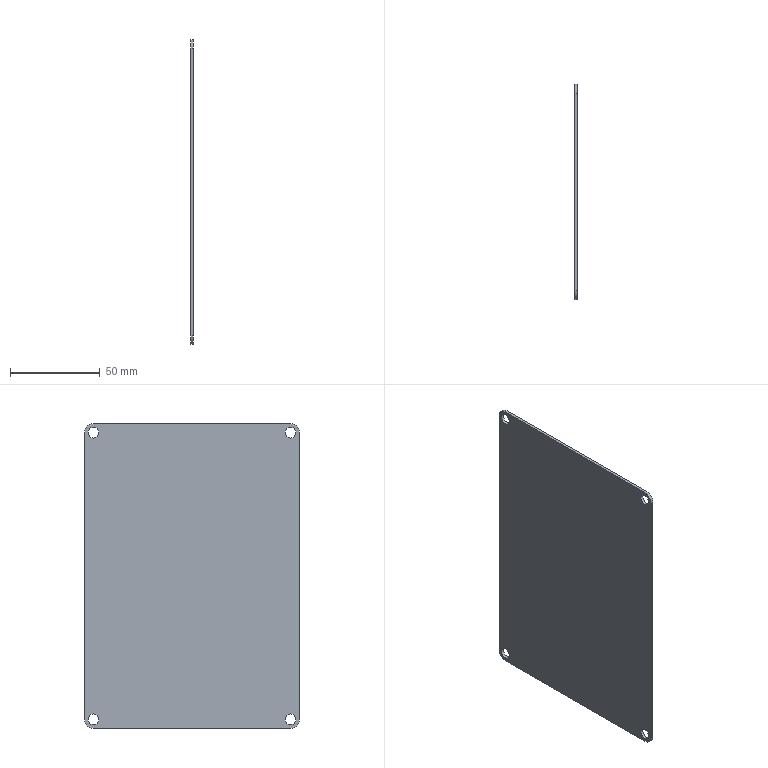Part | SolidWorks | 1 solid | 18 faces | box 1.5 x 120 x 170 mm | volume 30398 mm3 | cylinder 12 | plane 6 | commonest cylinder face diameters 6 x8 10 x4
STEP:
#1=CARTESIAN_POINT('',(-1.5,-55.,77.));
#2=VERTEX_POINT('',#1);
#3=CARTESIAN_POINT('',(-1.5,-55.,83.));
#4=VERTEX_POINT('',#3);
#5=CARTESIAN_POINT('',(-1.5,-55.,80.));
#6=DIRECTION('',(-1.,0.,0.));
#7=DIRECTION('',(0.,0.,-1.));
#8=AXIS2_PLACEMENT_3D('',#5,#6,#7);
#9=CIRCLE('',#8,3.);
#10=EDGE_CURVE('',#2,#4,#9,.T.);
#11=ORIENTED_EDGE('',*,*,#10,.T.);
#12=CARTESIAN_POINT('',(0.,-55.,83.));
#13=VERTEX_POINT('',#12);
#14=CARTESIAN_POINT('',(-1.501,-55.,83.));
#15=DIRECTION('',(1.,0.,0.));
#16=VECTOR('',#15,1000.);
#17=LINE('',#14,#16);
#18=EDGE_CURVE('',#4,#13,#17,.T.);
#19=ORIENTED_EDGE('',*,*,#18,.T.);
#20=CARTESIAN_POINT('',(0.,-55.,77.));
#21=VERTEX_POINT('',#20);
#22=CARTESIAN_POINT('',(0.,-55.,80.));
#23=DIRECTION('',(1.,0.,0.));
#24=DIRECTION('',(0.,0.,-1.));
#25=AXIS2_PLACEMENT_3D('',#22,#23,#24);
#26=CIRCLE('',#25,3.);
#27=EDGE_CURVE('',#13,#21,#26,.T.);
#28=ORIENTED_EDGE('',*,*,#27,.T.);
#29=CARTESIAN_POINT('',(-1.501,-55.,77.));
#30=DIRECTION('',(1.,0.,0.));
#31=VECTOR('',#30,1000.);
#32=LINE('',#29,#31);
#33=EDGE_CURVE('',#2,#21,#32,.T.);
#34=ORIENTED_EDGE('',*,*,#33,.F.);
#35=EDGE_LOOP('',(#11,#19,#28,#34));
#36=FACE_OUTER_BOUND('',#35,.T.);
#37=CARTESIAN_POINT('',(-1.501,-55.,80.));
#38=DIRECTION('',(1.,0.,0.));
#39=DIRECTION('',(0.,0.,-1.));
#40=AXIS2_PLACEMENT_3D('',#37,#38,#39);
#41=CYLINDRICAL_SURFACE('',#40,3.);
#42=ADVANCED_FACE('',(#36),#41,.F.);
#43=CARTESIAN_POINT('',(-1.5,-55.,-83.));
#44=VERTEX_POINT('',#43);
#45=CARTESIAN_POINT('',(-1.5,-55.,-77.));
#46=VERTEX_POINT('',#45);
#47=CARTESIAN_POINT('',(-1.5,-55.,-80.));
#48=DIRECTION('',(-1.,0.,0.));
#49=DIRECTION('',(0.,0.,-1.));
#50=AXIS2_PLACEMENT_3D('',#47,#48,#49);
#51=CIRCLE('',#50,3.);
#52=EDGE_CURVE('',#44,#46,#51,.T.);
#53=ORIENTED_EDGE('',*,*,#52,.T.);
#54=CARTESIAN_POINT('',(0.,-55.,-77.));
#55=VERTEX_POINT('',#54);
#56=CARTESIAN_POINT('',(-1.501,-55.,-77.));
#57=DIRECTION('',(1.,0.,0.));
#58=VECTOR('',#57,1000.);
#59=LINE('',#56,#58);
#60=EDGE_CURVE('',#46,#55,#59,.T.);
#61=ORIENTED_EDGE('',*,*,#60,.T.);
#62=CARTESIAN_POINT('',(0.,-55.,-83.));
#63=VERTEX_POINT('',#62);
#64=CARTESIAN_POINT('',(0.,-55.,-80.));
#65=DIRECTION('',(1.,0.,0.));
#66=DIRECTION('',(0.,0.,-1.));
#67=AXIS2_PLACEMENT_3D('',#64,#65,#66);
#68=CIRCLE('',#67,3.);
#69=EDGE_CURVE('',#55,#63,#68,.T.);
#70=ORIENTED_EDGE('',*,*,#69,.T.);
#71=CARTESIAN_POINT('',(-1.501,-55.,-83.));
#72=DIRECTION('',(1.,0.,0.));
#73=VECTOR('',#72,1000.);
#74=LINE('',#71,#73);
#75=EDGE_CURVE('',#44,#63,#74,.T.);
#76=ORIENTED_EDGE('',*,*,#75,.F.);
#77=EDGE_LOOP('',(#53,#61,#70,#76));
#78=FACE_OUTER_BOUND('',#77,.T.);
#79=CARTESIAN_POINT('',(-1.501,-55.,-80.));
#80=DIRECTION('',(1.,0.,0.));
#81=DIRECTION('',(0.,0.,-1.));
#82=AXIS2_PLACEMENT_3D('',#79,#80,#81);
#83=CYLINDRICAL_SURFACE('',#82,3.);
#84=ADVANCED_FACE('',(#78),#83,.F.);
#85=CARTESIAN_POINT('',(-1.5,55.,-83.));
#86=VERTEX_POINT('',#85);
#87=CARTESIAN_POINT('',(-1.5,55.,-77.));
#88=VERTEX_POINT('',#87);
#89=CARTESIAN_POINT('',(-1.5,55.,-80.));
#90=DIRECTION('',(-1.,0.,0.));
#91=DIRECTION('',(0.,0.,-1.));
#92=AXIS2_PLACEMENT_3D('',#89,#90,#91);
#93=CIRCLE('',#92,3.);
#94=EDGE_CURVE('',#86,#88,#93,.T.);
#95=ORIENTED_EDGE('',*,*,#94,.T.);
#96=CARTESIAN_POINT('',(0.,55.,-77.));
#97=VERTEX_POINT('',#96);
#98=CARTESIAN_POINT('',(-1.501,55.,-77.));
#99=DIRECTION('',(1.,0.,0.));
#100=VECTOR('',#99,1000.);
#101=LINE('',#98,#100);
#102=EDGE_CURVE('',#88,#97,#101,.T.);
#103=ORIENTED_EDGE('',*,*,#102,.T.);
#104=CARTESIAN_POINT('',(0.,55.,-83.));
#105=VERTEX_POINT('',#104);
#106=CARTESIAN_POINT('',(0.,55.,-80.));
#107=DIRECTION('',(1.,0.,0.));
#108=DIRECTION('',(0.,0.,-1.));
#109=AXIS2_PLACEMENT_3D('',#106,#107,#108);
#110=CIRCLE('',#109,3.);
#111=EDGE_CURVE('',#97,#105,#110,.T.);
#112=ORIENTED_EDGE('',*,*,#111,.T.);
#113=CARTESIAN_POINT('',(-1.501,55.,-83.));
#114=DIRECTION('',(1.,0.,0.));
#115=VECTOR('',#114,1000.);
#116=LINE('',#113,#115);
#117=EDGE_CURVE('',#86,#105,#116,.T.);
#118=ORIENTED_EDGE('',*,*,#117,.F.);
#119=EDGE_LOOP('',(#95,#103,#112,#118));
#120=FACE_OUTER_BOUND('',#119,.T.);
#121=CARTESIAN_POINT('',(-1.501,55.,-80.));
#122=DIRECTION('',(1.,0.,0.));
#123=DIRECTION('',(0.,0.,-1.));
#124=AXIS2_PLACEMENT_3D('',#121,#122,#123);
#125=CYLINDRICAL_SURFACE('',#124,3.);
#126=ADVANCED_FACE('',(#120),#125,.F.);
#127=CARTESIAN_POINT('',(-1.5,55.,77.));
#128=VERTEX_POINT('',#127);
#129=CARTESIAN_POINT('',(-1.5,55.,83.));
#130=VERTEX_POINT('',#129);
#131=CARTESIAN_POINT('',(-1.5,55.,80.));
#132=DIRECTION('',(-1.,0.,0.));
#133=DIRECTION('',(0.,0.,-1.));
#134=AXIS2_PLACEMENT_3D('',#131,#132,#133);
#135=CIRCLE('',#134,3.);
#136=EDGE_CURVE('',#128,#130,#135,.T.);
#137=ORIENTED_EDGE('',*,*,#136,.T.);
#138=CARTESIAN_POINT('',(0.,55.,83.));
#139=VERTEX_POINT('',#138);
#140=CARTESIAN_POINT('',(-1.501,55.,83.));
#141=DIRECTION('',(1.,0.,0.));
#142=VECTOR('',#141,1000.);
#143=LINE('',#140,#142);
#144=EDGE_CURVE('',#130,#139,#143,.T.);
#145=ORIENTED_EDGE('',*,*,#144,.T.);
#146=CARTESIAN_POINT('',(0.,55.,77.));
#147=VERTEX_POINT('',#146);
#148=CARTESIAN_POINT('',(0.,55.,80.));
#149=DIRECTION('',(1.,0.,0.));
#150=DIRECTION('',(0.,0.,-1.));
#151=AXIS2_PLACEMENT_3D('',#148,#149,#150);
#152=CIRCLE('',#151,3.);
#153=EDGE_CURVE('',#139,#147,#152,.T.);
#154=ORIENTED_EDGE('',*,*,#153,.T.);
#155=CARTESIAN_POINT('',(-1.501,55.,77.));
#156=DIRECTION('',(1.,0.,0.));
#157=VECTOR('',#156,1000.);
#158=LINE('',#155,#157);
#159=EDGE_CURVE('',#128,#147,#158,.T.);
#160=ORIENTED_EDGE('',*,*,#159,.F.);
#161=EDGE_LOOP('',(#137,#145,#154,#160));
#162=FACE_OUTER_BOUND('',#161,.T.);
#163=CARTESIAN_POINT('',(-1.501,55.,80.));
#164=DIRECTION('',(1.,0.,0.));
#165=DIRECTION('',(0.,0.,-1.));
#166=AXIS2_PLACEMENT_3D('',#163,#164,#165);
#167=CYLINDRICAL_SURFACE('',#166,3.);
#168=ADVANCED_FACE('',(#162),#167,.F.);
#169=CARTESIAN_POINT('',(-1.5,55.,85.));
#170=VERTEX_POINT('',#169);
#171=CARTESIAN_POINT('',(-1.5,-55.,85.));
#172=VERTEX_POINT('',#171);
#173=CARTESIAN_POINT('',(-1.5,-60.,85.));
#174=DIRECTION('',(0.,-1.,0.));
#175=VECTOR('',#174,1000.);
#176=LINE('',#173,#175);
#177=EDGE_CURVE('',#170,#172,#176,.T.);
#178=ORIENTED_EDGE('',*,*,#177,.T.);
#179=CARTESIAN_POINT('',(0.,-55.,85.));
#180=VERTEX_POINT('',#179);
#181=CARTESIAN_POINT('',(-1.5,-55.,85.));
#182=DIRECTION('',(1.,0.,0.));
#183=VECTOR('',#182,1000.);
#184=LINE('',#181,#183);
#185=EDGE_CURVE('',#172,#180,#184,.T.);
#186=ORIENTED_EDGE('',*,*,#185,.T.);
#187=CARTESIAN_POINT('',(0.,55.,85.));
#188=VERTEX_POINT('',#187);
#189=CARTESIAN_POINT('',(0.,-60.,85.));
#190=DIRECTION('',(0.,-1.,0.));
#191=VECTOR('',#190,1000.);
#192=LINE('',#189,#191);
#193=EDGE_CURVE('',#188,#180,#192,.T.);
#194=ORIENTED_EDGE('',*,*,#193,.F.);
#195=CARTESIAN_POINT('',(-1.5,55.,85.));
#196=DIRECTION('',(-1.,0.,0.));
#197=VECTOR('',#196,1000.);
#198=LINE('',#195,#197);
#199=EDGE_CURVE('',#188,#170,#198,.T.);
#200=ORIENTED_EDGE('',*,*,#199,.T.);
#201=EDGE_LOOP('',(#178,#186,#194,#200));
#202=FACE_OUTER_BOUND('',#201,.T.);
#203=CARTESIAN_POINT('',(-1.5,-60.,85.));
#204=DIRECTION('',(0.,0.,1.));
#205=DIRECTION('',(0.,-1.,0.));
#206=AXIS2_PLACEMENT_3D('',#203,#204,#205);
#207=PLANE('',#206);
#208=ADVANCED_FACE('',(#202),#207,.T.);
#209=CARTESIAN_POINT('',(0.,60.,-80.));
#210=VERTEX_POINT('',#209);
#211=CARTESIAN_POINT('',(0.,60.,80.));
#212=VERTEX_POINT('',#211);
#213=CARTESIAN_POINT('',(0.,60.,-85.));
#214=DIRECTION('',(0.,0.,1.));
#215=VECTOR('',#214,1000.);
#216=LINE('',#213,#215);
#217=EDGE_CURVE('',#210,#212,#216,.T.);
#218=ORIENTED_EDGE('',*,*,#217,.F.);
#219=CARTESIAN_POINT('',(-1.5,60.,-80.));
#220=VERTEX_POINT('',#219);
#221=CARTESIAN_POINT('',(-1.5,60.,-80.));
#222=DIRECTION('',(-1.,0.,0.));
#223=VECTOR('',#222,1000.);
#224=LINE('',#221,#223);
#225=EDGE_CURVE('',#210,#220,#224,.T.);
#226=ORIENTED_EDGE('',*,*,#225,.T.);
#227=CARTESIAN_POINT('',(-1.5,60.,80.));
#228=VERTEX_POINT('',#227);
#229=CARTESIAN_POINT('',(-1.5,60.,-85.));
#230=DIRECTION('',(0.,0.,1.));
#231=VECTOR('',#230,1000.);
#232=LINE('',#229,#231);
#233=EDGE_CURVE('',#220,#228,#232,.T.);
#234=ORIENTED_EDGE('',*,*,#233,.T.);
#235=CARTESIAN_POINT('',(-1.5,60.,80.));
#236=DIRECTION('',(1.,0.,0.));
#237=VECTOR('',#236,1000.);
#238=LINE('',#235,#237);
#239=EDGE_CURVE('',#228,#212,#238,.T.);
#240=ORIENTED_EDGE('',*,*,#239,.T.);
#241=EDGE_LOOP('',(#218,#226,#234,#240));
#242=FACE_OUTER_BOUND('',#241,.T.);
#243=CARTESIAN_POINT('',(-1.5,60.,-85.));
#244=DIRECTION('',(0.,1.,0.));
#245=DIRECTION('',(0.,0.,1.));
#246=AXIS2_PLACEMENT_3D('',#243,#244,#245);
#247=PLANE('',#246);
#248=ADVANCED_FACE('',(#242),#247,.T.);
#249=CARTESIAN_POINT('',(0.,-55.,-85.));
#250=VERTEX_POINT('',#249);
#251=CARTESIAN_POINT('',(0.,55.,-85.));
#252=VERTEX_POINT('',#251);
#253=CARTESIAN_POINT('',(0.,-60.,-85.));
#254=DIRECTION('',(0.,1.,0.));
#255=VECTOR('',#254,1000.);
#256=LINE('',#253,#255);
#257=EDGE_CURVE('',#250,#252,#256,.T.);
#258=ORIENTED_EDGE('',*,*,#257,.F.);
#259=CARTESIAN_POINT('',(-1.5,-55.,-85.));
#260=VERTEX_POINT('',#259);
#261=CARTESIAN_POINT('',(-1.5,-55.,-85.));
#262=DIRECTION('',(-1.,0.,0.));
#263=VECTOR('',#262,1000.);
#264=LINE('',#261,#263);
#265=EDGE_CURVE('',#250,#260,#264,.T.);
#266=ORIENTED_EDGE('',*,*,#265,.T.);
#267=CARTESIAN_POINT('',(-1.5,55.,-85.));
#268=VERTEX_POINT('',#267);
#269=CARTESIAN_POINT('',(-1.5,-60.,-85.));
#270=DIRECTION('',(0.,1.,0.));
#271=VECTOR('',#270,1000.);
#272=LINE('',#269,#271);
#273=EDGE_CURVE('',#260,#268,#272,.T.);
#274=ORIENTED_EDGE('',*,*,#273,.T.);
#275=CARTESIAN_POINT('',(-1.5,55.,-85.));
#276=DIRECTION('',(1.,0.,0.));
#277=VECTOR('',#276,1000.);
#278=LINE('',#275,#277);
#279=EDGE_CURVE('',#268,#252,#278,.T.);
#280=ORIENTED_EDGE('',*,*,#279,.T.);
#281=EDGE_LOOP('',(#258,#266,#274,#280));
#282=FACE_OUTER_BOUND('',#281,.T.);
#283=CARTESIAN_POINT('',(-1.5,-60.,-85.));
#284=DIRECTION('',(0.,0.,-1.));
#285=DIRECTION('',(-1.,0.,0.));
#286=AXIS2_PLACEMENT_3D('',#283,#284,#285);
#287=PLANE('',#286);
#288=ADVANCED_FACE('',(#282),#287,.T.);
#289=CARTESIAN_POINT('',(0.,-60.,80.));
#290=VERTEX_POINT('',#289);
#291=CARTESIAN_POINT('',(0.,-60.,-80.));
#292=VERTEX_POINT('',#291);
#293=CARTESIAN_POINT('',(0.,-60.,-85.));
#294=DIRECTION('',(0.,0.,-1.));
#295=VECTOR('',#294,1000.);
#296=LINE('',#293,#295);
#297=EDGE_CURVE('',#290,#292,#296,.T.);
#298=ORIENTED_EDGE('',*,*,#297,.F.);
#299=CARTESIAN_POINT('',(-1.5,-60.,80.));
#300=VERTEX_POINT('',#299);
#301=CARTESIAN_POINT('',(-1.5,-60.,80.));
#302=DIRECTION('',(-1.,0.,0.));
#303=VECTOR('',#302,1000.);
#304=LINE('',#301,#303);
#305=EDGE_CURVE('',#290,#300,#304,.T.);
#306=ORIENTED_EDGE('',*,*,#305,.T.);
#307=CARTESIAN_POINT('',(-1.5,-60.,-80.));
#308=VERTEX_POINT('',#307);
#309=CARTESIAN_POINT('',(-1.5,-60.,-85.));
#310=DIRECTION('',(0.,0.,-1.));
#311=VECTOR('',#310,1000.);
#312=LINE('',#309,#311);
#313=EDGE_CURVE('',#300,#308,#312,.T.);
#314=ORIENTED_EDGE('',*,*,#313,.T.);
#315=CARTESIAN_POINT('',(-1.5,-60.,-80.));
#316=DIRECTION('',(1.,0.,0.));
#317=VECTOR('',#316,1000.);
#318=LINE('',#315,#317);
#319=EDGE_CURVE('',#308,#292,#318,.T.);
#320=ORIENTED_EDGE('',*,*,#319,.T.);
#321=EDGE_LOOP('',(#298,#306,#314,#320));
#322=FACE_OUTER_BOUND('',#321,.T.);
#323=CARTESIAN_POINT('',(-1.5,-60.,-85.));
#324=DIRECTION('',(0.,-1.,0.));
#325=DIRECTION('',(0.,0.,-1.));
#326=AXIS2_PLACEMENT_3D('',#323,#324,#325);
#327=PLANE('',#326);
#328=ADVANCED_FACE('',(#322),#327,.T.);
#329=ORIENTED_EDGE('',*,*,#10,.F.);
#330=CARTESIAN_POINT('',(-1.5,-55.,80.));
#331=DIRECTION('',(-1.,0.,0.));
#332=DIRECTION('',(0.,0.,-1.));
#333=AXIS2_PLACEMENT_3D('',#330,#331,#332);
#334=CIRCLE('',#333,3.);
#335=EDGE_CURVE('',#4,#2,#334,.T.);
#336=ORIENTED_EDGE('',*,*,#335,.F.);
#337=EDGE_LOOP('',(#329,#336));
#338=FACE_BOUND('',#337,.T.);
#339=ORIENTED_EDGE('',*,*,#52,.F.);
#340=CARTESIAN_POINT('',(-1.5,-55.,-80.));
#341=DIRECTION('',(-1.,0.,0.));
#342=DIRECTION('',(0.,0.,-1.));
#343=AXIS2_PLACEMENT_3D('',#340,#341,#342);
#344=CIRCLE('',#343,3.);
#345=EDGE_CURVE('',#46,#44,#344,.T.);
#346=ORIENTED_EDGE('',*,*,#345,.F.);
#347=EDGE_LOOP('',(#339,#346));
#348=FACE_BOUND('',#347,.T.);
#349=ORIENTED_EDGE('',*,*,#94,.F.);
#350=CARTESIAN_POINT('',(-1.5,55.,-80.));
#351=DIRECTION('',(-1.,0.,0.));
#352=DIRECTION('',(0.,0.,-1.));
#353=AXIS2_PLACEMENT_3D('',#350,#351,#352);
#354=CIRCLE('',#353,3.);
#355=EDGE_CURVE('',#88,#86,#354,.T.);
#356=ORIENTED_EDGE('',*,*,#355,.F.);
#357=EDGE_LOOP('',(#349,#356));
#358=FACE_BOUND('',#357,.T.);
#359=ORIENTED_EDGE('',*,*,#136,.F.);
#360=CARTESIAN_POINT('',(-1.5,55.,80.));
#361=DIRECTION('',(-1.,0.,0.));
#362=DIRECTION('',(0.,0.,-1.));
#363=AXIS2_PLACEMENT_3D('',#360,#361,#362);
#364=CIRCLE('',#363,3.);
#365=EDGE_CURVE('',#130,#128,#364,.T.);
#366=ORIENTED_EDGE('',*,*,#365,.F.);
#367=EDGE_LOOP('',(#359,#366));
#368=FACE_BOUND('',#367,.T.);
#369=ORIENTED_EDGE('',*,*,#313,.F.);
#370=CARTESIAN_POINT('',(-1.5,-55.,80.));
#371=DIRECTION('',(-1.,0.,0.));
#372=DIRECTION('',(0.,0.,-1.));
#373=AXIS2_PLACEMENT_3D('',#370,#371,#372);
#374=CIRCLE('',#373,5.);
#375=EDGE_CURVE('',#300,#172,#374,.T.);
#376=ORIENTED_EDGE('',*,*,#375,.T.);
#377=ORIENTED_EDGE('',*,*,#177,.F.);
#378=CARTESIAN_POINT('',(-1.5,55.,80.));
#379=DIRECTION('',(-1.,0.,0.));
#380=DIRECTION('',(0.,0.,-1.));
#381=AXIS2_PLACEMENT_3D('',#378,#379,#380);
#382=CIRCLE('',#381,5.);
#383=EDGE_CURVE('',#170,#228,#382,.T.);
#384=ORIENTED_EDGE('',*,*,#383,.T.);
#385=ORIENTED_EDGE('',*,*,#233,.F.);
#386=CARTESIAN_POINT('',(-1.5,55.,-80.));
#387=DIRECTION('',(-1.,0.,0.));
#388=DIRECTION('',(0.,0.,-1.));
#389=AXIS2_PLACEMENT_3D('',#386,#387,#388);
#390=CIRCLE('',#389,5.);
#391=EDGE_CURVE('',#220,#268,#390,.T.);
#392=ORIENTED_EDGE('',*,*,#391,.T.);
#393=ORIENTED_EDGE('',*,*,#273,.F.);
#394=CARTESIAN_POINT('',(-1.5,-55.,-80.));
#395=DIRECTION('',(-1.,0.,0.));
#396=DIRECTION('',(0.,0.,-1.));
#397=AXIS2_PLACEMENT_3D('',#394,#395,#396);
#398=CIRCLE('',#397,5.);
#399=EDGE_CURVE('',#260,#308,#398,.T.);
#400=ORIENTED_EDGE('',*,*,#399,.T.);
#401=EDGE_LOOP('',(#369,#376,#377,#384,#385,#392,#393,#400));
#402=FACE_OUTER_BOUND('',#401,.T.);
#403=CARTESIAN_POINT('',(-1.5,0.,0.));
#404=DIRECTION('',(1.,0.,0.));
#405=DIRECTION('',(0.,0.,-1.));
#406=AXIS2_PLACEMENT_3D('',#403,#404,#405);
#407=PLANE('',#406);
#408=ADVANCED_FACE('',(#338,#348,#358,#368,#402),#407,.F.);
#409=CARTESIAN_POINT('',(0.,-55.,80.));
#410=DIRECTION('',(1.,0.,0.));
#411=DIRECTION('',(0.,0.,-1.));
#412=AXIS2_PLACEMENT_3D('',#409,#410,#411);
#413=CIRCLE('',#412,3.);
#414=EDGE_CURVE('',#21,#13,#413,.T.);
#415=ORIENTED_EDGE('',*,*,#414,.F.);
#416=ORIENTED_EDGE('',*,*,#27,.F.);
#417=EDGE_LOOP('',(#415,#416));
#418=FACE_BOUND('',#417,.T.);
#419=CARTESIAN_POINT('',(0.,-55.,-80.));
#420=DIRECTION('',(1.,0.,0.));
#421=DIRECTION('',(0.,0.,-1.));
#422=AXIS2_PLACEMENT_3D('',#419,#420,#421);
#423=CIRCLE('',#422,3.);
#424=EDGE_CURVE('',#63,#55,#423,.T.);
#425=ORIENTED_EDGE('',*,*,#424,.F.);
#426=ORIENTED_EDGE('',*,*,#69,.F.);
#427=EDGE_LOOP('',(#425,#426));
#428=FACE_BOUND('',#427,.T.);
#429=CARTESIAN_POINT('',(0.,55.,-80.));
#430=DIRECTION('',(1.,0.,0.));
#431=DIRECTION('',(0.,0.,-1.));
#432=AXIS2_PLACEMENT_3D('',#429,#430,#431);
#433=CIRCLE('',#432,3.);
#434=EDGE_CURVE('',#105,#97,#433,.T.);
#435=ORIENTED_EDGE('',*,*,#434,.F.);
#436=ORIENTED_EDGE('',*,*,#111,.F.);
#437=EDGE_LOOP('',(#435,#436));
#438=FACE_BOUND('',#437,.T.);
#439=CARTESIAN_POINT('',(0.,55.,80.));
#440=DIRECTION('',(1.,0.,0.));
#441=DIRECTION('',(0.,0.,-1.));
#442=AXIS2_PLACEMENT_3D('',#439,#440,#441);
#443=CIRCLE('',#442,3.);
#444=EDGE_CURVE('',#147,#139,#443,.T.);
#445=ORIENTED_EDGE('',*,*,#444,.F.);
#446=ORIENTED_EDGE('',*,*,#153,.F.);
#447=EDGE_LOOP('',(#445,#446));
#448=FACE_BOUND('',#447,.T.);
#449=ORIENTED_EDGE('',*,*,#193,.T.);
#450=CARTESIAN_POINT('',(0.,-55.,80.));
#451=DIRECTION('',(1.,0.,0.));
#452=DIRECTION('',(0.,0.,-1.));
#453=AXIS2_PLACEMENT_3D('',#450,#451,#452);
#454=CIRCLE('',#453,5.);
#455=EDGE_CURVE('',#180,#290,#454,.T.);
#456=ORIENTED_EDGE('',*,*,#455,.T.);
#457=ORIENTED_EDGE('',*,*,#297,.T.);
#458=CARTESIAN_POINT('',(0.,-55.,-80.));
#459=DIRECTION('',(1.,0.,0.));
#460=DIRECTION('',(0.,0.,-1.));
#461=AXIS2_PLACEMENT_3D('',#458,#459,#460);
#462=CIRCLE('',#461,5.);
#463=EDGE_CURVE('',#292,#250,#462,.T.);
#464=ORIENTED_EDGE('',*,*,#463,.T.);
#465=ORIENTED_EDGE('',*,*,#257,.T.);
#466=CARTESIAN_POINT('',(0.,55.,-80.));
#467=DIRECTION('',(1.,0.,0.));
#468=DIRECTION('',(0.,0.,-1.));
#469=AXIS2_PLACEMENT_3D('',#466,#467,#468);
#470=CIRCLE('',#469,5.);
#471=EDGE_CURVE('',#252,#210,#470,.T.);
#472=ORIENTED_EDGE('',*,*,#471,.T.);
#473=ORIENTED_EDGE('',*,*,#217,.T.);
#474=CARTESIAN_POINT('',(0.,55.,80.));
#475=DIRECTION('',(1.,0.,0.));
#476=DIRECTION('',(0.,0.,-1.));
#477=AXIS2_PLACEMENT_3D('',#474,#475,#476);
#478=CIRCLE('',#477,5.);
#479=EDGE_CURVE('',#212,#188,#478,.T.);
#480=ORIENTED_EDGE('',*,*,#479,.T.);
#481=EDGE_LOOP('',(#449,#456,#457,#464,#465,#472,#473,#480));
#482=FACE_OUTER_BOUND('',#481,.T.);
#483=CARTESIAN_POINT('',(0.,0.,0.));
#484=DIRECTION('',(1.,0.,0.));
#485=DIRECTION('',(0.,0.,-1.));
#486=AXIS2_PLACEMENT_3D('',#483,#484,#485);
#487=PLANE('',#486);
#488=ADVANCED_FACE('',(#418,#428,#438,#448,#482),#487,.T.);
#489=ORIENTED_EDGE('',*,*,#375,.F.);
#490=ORIENTED_EDGE('',*,*,#305,.F.);
#491=ORIENTED_EDGE('',*,*,#455,.F.);
#492=ORIENTED_EDGE('',*,*,#185,.F.);
#493=EDGE_LOOP('',(#489,#490,#491,#492));
#494=FACE_OUTER_BOUND('',#493,.T.);
#495=CARTESIAN_POINT('',(-1.5,-55.,80.));
#496=DIRECTION('',(1.,0.,0.));
#497=DIRECTION('',(0.,0.,-1.));
#498=AXIS2_PLACEMENT_3D('',#495,#496,#497);
#499=CYLINDRICAL_SURFACE('',#498,5.);
#500=ADVANCED_FACE('',(#494),#499,.T.);
#501=ORIENTED_EDGE('',*,*,#399,.F.);
#502=ORIENTED_EDGE('',*,*,#265,.F.);
#503=ORIENTED_EDGE('',*,*,#463,.F.);
#504=ORIENTED_EDGE('',*,*,#319,.F.);
#505=EDGE_LOOP('',(#501,#502,#503,#504));
#506=FACE_OUTER_BOUND('',#505,.T.);
#507=CARTESIAN_POINT('',(-1.5,-55.,-80.));
#508=DIRECTION('',(1.,0.,0.));
#509=DIRECTION('',(0.,0.,-1.));
#510=AXIS2_PLACEMENT_3D('',#507,#508,#509);
#511=CYLINDRICAL_SURFACE('',#510,5.);
#512=ADVANCED_FACE('',(#506),#511,.T.);
#513=ORIENTED_EDGE('',*,*,#391,.F.);
#514=ORIENTED_EDGE('',*,*,#225,.F.);
#515=ORIENTED_EDGE('',*,*,#471,.F.);
#516=ORIENTED_EDGE('',*,*,#279,.F.);
#517=EDGE_LOOP('',(#513,#514,#515,#516));
#518=FACE_OUTER_BOUND('',#517,.T.);
#519=CARTESIAN_POINT('',(-1.5,55.,-80.));
#520=DIRECTION('',(1.,0.,0.));
#521=DIRECTION('',(0.,0.,-1.));
#522=AXIS2_PLACEMENT_3D('',#519,#520,#521);
#523=CYLINDRICAL_SURFACE('',#522,5.);
#524=ADVANCED_FACE('',(#518),#523,.T.);
#525=ORIENTED_EDGE('',*,*,#383,.F.);
#526=ORIENTED_EDGE('',*,*,#199,.F.);
#527=ORIENTED_EDGE('',*,*,#479,.F.);
#528=ORIENTED_EDGE('',*,*,#239,.F.);
#529=EDGE_LOOP('',(#525,#526,#527,#528));
#530=FACE_OUTER_BOUND('',#529,.T.);
#531=CARTESIAN_POINT('',(-1.5,55.,80.));
#532=DIRECTION('',(1.,0.,0.));
#533=DIRECTION('',(0.,0.,-1.));
#534=AXIS2_PLACEMENT_3D('',#531,#532,#533);
#535=CYLINDRICAL_SURFACE('',#534,5.);
#536=ADVANCED_FACE('',(#530),#535,.T.);
#537=ORIENTED_EDGE('',*,*,#144,.F.);
#538=ORIENTED_EDGE('',*,*,#365,.T.);
#539=ORIENTED_EDGE('',*,*,#159,.T.);
#540=ORIENTED_EDGE('',*,*,#444,.T.);
#541=EDGE_LOOP('',(#537,#538,#539,#540));
#542=FACE_OUTER_BOUND('',#541,.T.);
#543=CARTESIAN_POINT('',(-1.501,55.,80.));
#544=DIRECTION('',(1.,0.,0.));
#545=DIRECTION('',(0.,0.,-1.));
#546=AXIS2_PLACEMENT_3D('',#543,#544,#545);
#547=CYLINDRICAL_SURFACE('',#546,3.);
#548=ADVANCED_FACE('',(#542),#547,.F.);
#549=ORIENTED_EDGE('',*,*,#102,.F.);
#550=ORIENTED_EDGE('',*,*,#355,.T.);
#551=ORIENTED_EDGE('',*,*,#117,.T.);
#552=ORIENTED_EDGE('',*,*,#434,.T.);
#553=EDGE_LOOP('',(#549,#550,#551,#552));
#554=FACE_OUTER_BOUND('',#553,.T.);
#555=CARTESIAN_POINT('',(-1.501,55.,-80.));
#556=DIRECTION('',(1.,0.,0.));
#557=DIRECTION('',(0.,0.,-1.));
#558=AXIS2_PLACEMENT_3D('',#555,#556,#557);
#559=CYLINDRICAL_SURFACE('',#558,3.);
#560=ADVANCED_FACE('',(#554),#559,.F.);
#561=ORIENTED_EDGE('',*,*,#60,.F.);
#562=ORIENTED_EDGE('',*,*,#345,.T.);
#563=ORIENTED_EDGE('',*,*,#75,.T.);
#564=ORIENTED_EDGE('',*,*,#424,.T.);
#565=EDGE_LOOP('',(#561,#562,#563,#564));
#566=FACE_OUTER_BOUND('',#565,.T.);
#567=CARTESIAN_POINT('',(-1.501,-55.,-80.));
#568=DIRECTION('',(1.,0.,0.));
#569=DIRECTION('',(0.,0.,-1.));
#570=AXIS2_PLACEMENT_3D('',#567,#568,#569);
#571=CYLINDRICAL_SURFACE('',#570,3.);
#572=ADVANCED_FACE('',(#566),#571,.F.);
#573=ORIENTED_EDGE('',*,*,#18,.F.);
#574=ORIENTED_EDGE('',*,*,#335,.T.);
#575=ORIENTED_EDGE('',*,*,#33,.T.);
#576=ORIENTED_EDGE('',*,*,#414,.T.);
#577=EDGE_LOOP('',(#573,#574,#575,#576));
#578=FACE_OUTER_BOUND('',#577,.T.);
#579=CARTESIAN_POINT('',(-1.501,-55.,80.));
#580=DIRECTION('',(1.,0.,0.));
#581=DIRECTION('',(0.,0.,-1.));
#582=AXIS2_PLACEMENT_3D('',#579,#580,#581);
#583=CYLINDRICAL_SURFACE('',#582,3.);
#584=ADVANCED_FACE('',(#578),#583,.F.);
#585=CLOSED_SHELL('',(#42,#84,#126,#168,#208,#248,#288,#328,#408,#488,#500,#512,#524,#536,#548,#560,#572,#584));
#586=MANIFOLD_SOLID_BREP('',#585);
#587=CARTESIAN_POINT('',(0.,0.,0.));
#588=DIRECTION('',(0.,0.,1.));
#589=DIRECTION('',(1.,0.,0.));
#590=AXIS2_PLACEMENT_3D('',#587,#588,#589);
#591=(LENGTH_UNIT()NAMED_UNIT(*)SI_UNIT(.MILLI.,.METRE.));
#592=UNCERTAINTY_MEASURE_WITH_UNIT(LENGTH_MEASURE(0.00001),#591,'','');
#593=(NAMED_UNIT(*)PLANE_ANGLE_UNIT()SI_UNIT($,.RADIAN.));
#594=(NAMED_UNIT(*)SI_UNIT($,.STERADIAN.)SOLID_ANGLE_UNIT());
#595=(GEOMETRIC_REPRESENTATION_CONTEXT(3)GLOBAL_UNCERTAINTY_ASSIGNED_CONTEXT((#592))GLOBAL_UNIT_ASSIGNED_CONTEXT((#591,#593,#594))REPRESENTATION_CONTEXT('',''));
#596=ADVANCED_BREP_SHAPE_REPRESENTATION('',(#586,#590),#595);